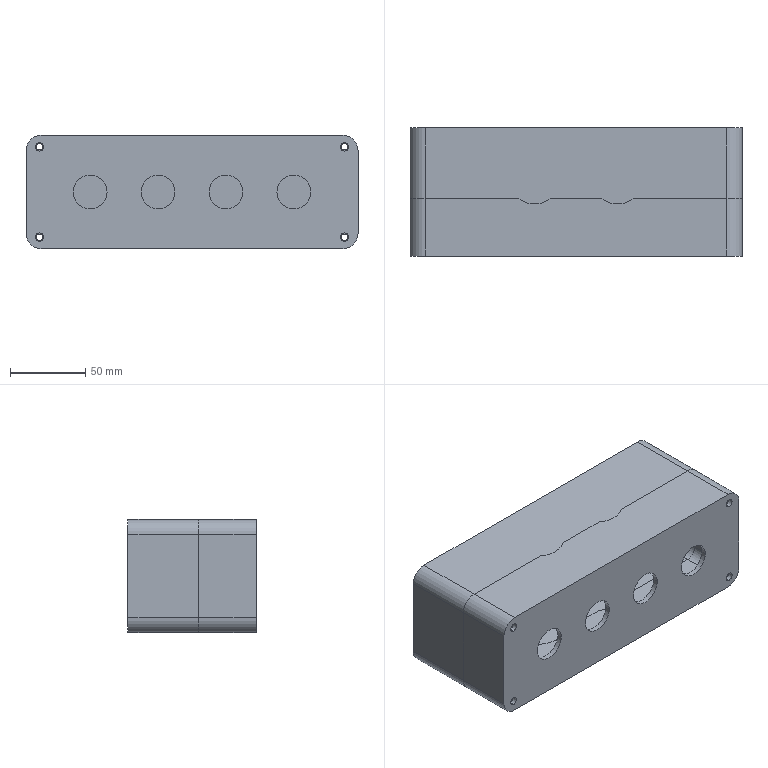Part | STEP file | four-hole button box TYX4 | 2 solids | 1182 faces | box 220 x 85 x 75 mm | volume 244482 mm3 | plane 780 | spline 338 | cylinder 64 | commonest cylinder face diameters 4.2 x8 5.5 x8 13.5 x8 20 x8 22.4 x8 34 x8